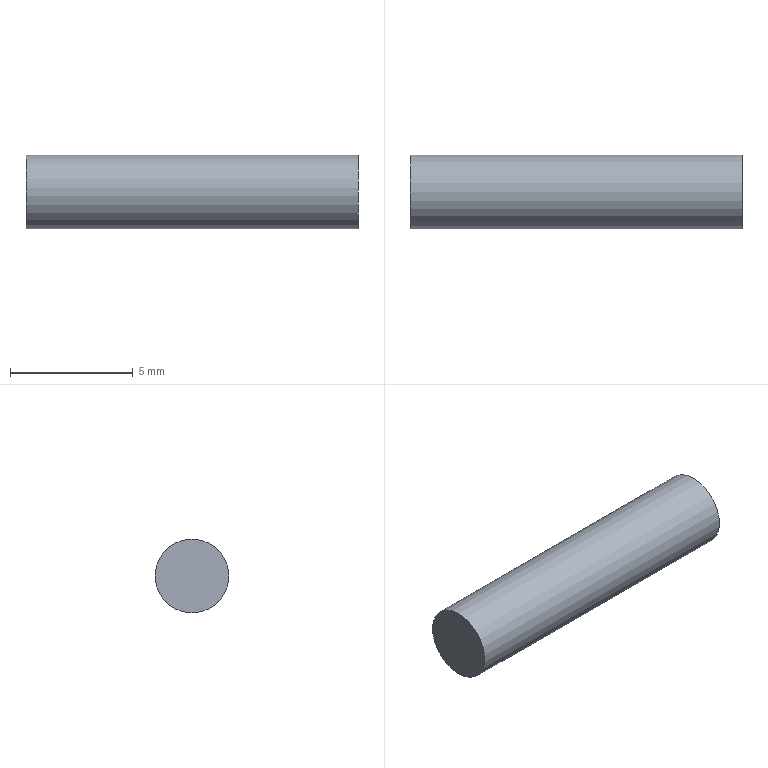Part | STEP file | solid 193 | 1 solid | 3 faces | box 13.5 x 3 x 3 mm | volume 95.426 mm3 | plane 2 | cylinder 1 | commonest cylinder face diameters 3 x1